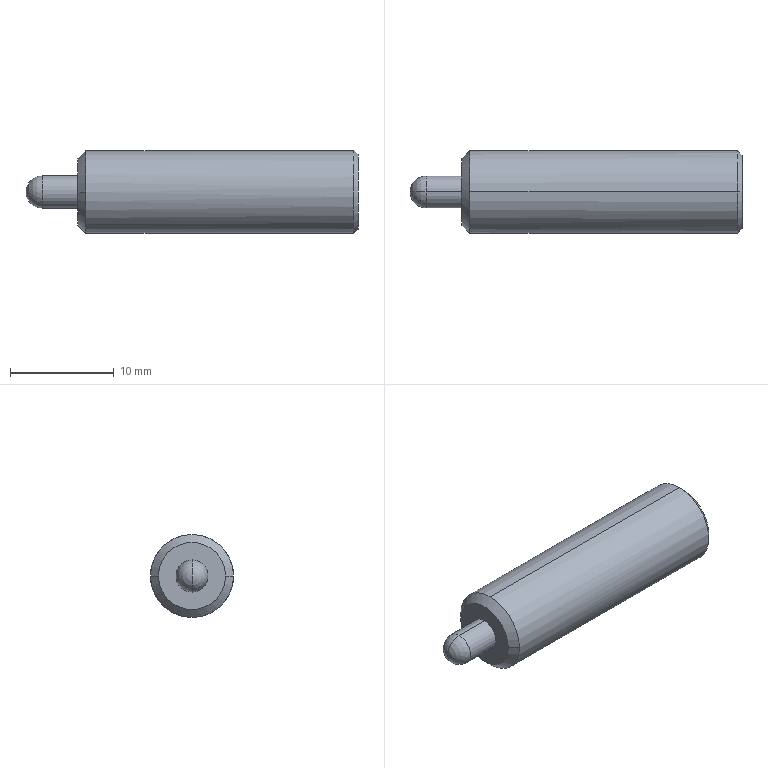Part | SolidWorks | features BaseBody 1 | 1 solid | 19 faces | box 32 x 8 x 8 mm | volume 1371 mm3 | plane 9 | cylinder 4 | cone 4 | sphere 2 | commonest cylinder face diameters 3.1 x2 8 x2
STEP:
#1=CARTESIAN_POINT('',(-3.45,0.,1.55));
#2=VERTEX_POINT('',#1);
#3=CARTESIAN_POINT('',(-3.45,0.,-1.55));
#4=VERTEX_POINT('',#3);
#5=CARTESIAN_POINT('',(-3.45,0.,0.));
#6=DIRECTION('',(1.,0.,0.));
#7=DIRECTION('',(0.,0.,-1.));
#8=AXIS2_PLACEMENT_3D('',#5,#6,#7);
#9=CIRCLE('',#8,1.55);
#10=EDGE_CURVE('',#2,#4,#9,.T.);
#11=ORIENTED_EDGE('',*,*,#10,.F.);
#12=CARTESIAN_POINT('',(-3.45,0.,0.));
#13=DIRECTION('',(0.,-1.,0.));
#14=DIRECTION('',(0.,0.,-1.));
#15=AXIS2_PLACEMENT_3D('',#12,#13,#14);
#16=CIRCLE('',#15,1.55);
#17=EDGE_CURVE('',#2,#4,#16,.T.);
#18=ORIENTED_EDGE('',*,*,#17,.T.);
#19=EDGE_LOOP('',(#11,#18));
#20=FACE_OUTER_BOUND('',#19,.T.);
#21=CARTESIAN_POINT('',(-3.45,0.,0.));
#22=DIRECTION('',(-1.,0.,0.));
#23=DIRECTION('',(0.,0.,-1.));
#24=AXIS2_PLACEMENT_3D('',#21,#22,#23);
#25=SPHERICAL_SURFACE('',#24,1.55);
#26=ADVANCED_FACE('',(#20),#25,.T.);
#27=CARTESIAN_POINT('',(27.,-0.7217,-1.25));
#28=VERTEX_POINT('',#27);
#29=CARTESIAN_POINT('',(25.,-0.7217,-1.25));
#30=VERTEX_POINT('',#29);
#31=CARTESIAN_POINT('',(25.,-0.7217,-1.25));
#32=DIRECTION('',(-1.,0.,0.));
#33=VECTOR('',#32,1000.);
#34=LINE('',#31,#33);
#35=EDGE_CURVE('',#28,#30,#34,.T.);
#36=ORIENTED_EDGE('',*,*,#35,.T.);
#37=CARTESIAN_POINT('',(25.,-1.443,0.));
#38=VERTEX_POINT('',#37);
#39=CARTESIAN_POINT('',(25.,-1.443,0.));
#40=DIRECTION('',(0.,0.5,-0.866));
#41=VECTOR('',#40,1000.);
#42=LINE('',#39,#41);
#43=EDGE_CURVE('',#38,#30,#42,.T.);
#44=ORIENTED_EDGE('',*,*,#43,.F.);
#45=CARTESIAN_POINT('',(27.,-1.443,0.));
#46=VERTEX_POINT('',#45);
#47=CARTESIAN_POINT('',(25.,-1.443,0.));
#48=DIRECTION('',(1.,0.,0.));
#49=VECTOR('',#48,1000.);
#50=LINE('',#47,#49);
#51=EDGE_CURVE('',#38,#46,#50,.T.);
#52=ORIENTED_EDGE('',*,*,#51,.T.);
#53=CARTESIAN_POINT('',(27.,-1.443,0.));
#54=DIRECTION('',(0.,-0.5,0.866));
#55=VECTOR('',#54,1000.);
#56=LINE('',#53,#55);
#57=EDGE_CURVE('',#28,#46,#56,.T.);
#58=ORIENTED_EDGE('',*,*,#57,.F.);
#59=EDGE_LOOP('',(#36,#44,#52,#58));
#60=FACE_OUTER_BOUND('',#59,.T.);
#61=CARTESIAN_POINT('',(25.,-1.443,0.));
#62=DIRECTION('',(0.,-0.866,-0.5));
#63=DIRECTION('',(0.,0.5,-0.866));
#64=AXIS2_PLACEMENT_3D('',#61,#62,#63);
#65=PLANE('',#64);
#66=ADVANCED_FACE('',(#60),#65,.F.);
#67=CARTESIAN_POINT('',(27.,0.7217,-1.25));
#68=VERTEX_POINT('',#67);
#69=CARTESIAN_POINT('',(25.,0.7217,-1.25));
#70=VERTEX_POINT('',#69);
#71=CARTESIAN_POINT('',(25.,0.7217,-1.25));
#72=DIRECTION('',(-1.,0.,0.));
#73=VECTOR('',#72,1000.);
#74=LINE('',#71,#73);
#75=EDGE_CURVE('',#68,#70,#74,.T.);
#76=ORIENTED_EDGE('',*,*,#75,.T.);
#77=CARTESIAN_POINT('',(25.,-0.7217,-1.25));
#78=DIRECTION('',(0.,1.,0.));
#79=VECTOR('',#78,1000.);
#80=LINE('',#77,#79);
#81=EDGE_CURVE('',#30,#70,#80,.T.);
#82=ORIENTED_EDGE('',*,*,#81,.F.);
#83=ORIENTED_EDGE('',*,*,#35,.F.);
#84=CARTESIAN_POINT('',(27.,-0.7217,-1.25));
#85=DIRECTION('',(0.,-1.,0.));
#86=VECTOR('',#85,1000.);
#87=LINE('',#84,#86);
#88=EDGE_CURVE('',#68,#28,#87,.T.);
#89=ORIENTED_EDGE('',*,*,#88,.F.);
#90=EDGE_LOOP('',(#76,#82,#83,#89));
#91=FACE_OUTER_BOUND('',#90,.T.);
#92=CARTESIAN_POINT('',(25.,-0.7217,-1.25));
#93=DIRECTION('',(0.,0.,-1.));
#94=DIRECTION('',(0.,-1.,0.));
#95=AXIS2_PLACEMENT_3D('',#92,#93,#94);
#96=PLANE('',#95);
#97=ADVANCED_FACE('',(#91),#96,.F.);
#98=ORIENTED_EDGE('',*,*,#51,.F.);
#99=CARTESIAN_POINT('',(25.,-0.7217,1.25));
#100=VERTEX_POINT('',#99);
#101=CARTESIAN_POINT('',(25.,-0.7217,1.25));
#102=DIRECTION('',(0.,-0.5,-0.866));
#103=VECTOR('',#102,1000.);
#104=LINE('',#101,#103);
#105=EDGE_CURVE('',#100,#38,#104,.T.);
#106=ORIENTED_EDGE('',*,*,#105,.F.);
#107=CARTESIAN_POINT('',(27.,-0.7217,1.25));
#108=VERTEX_POINT('',#107);
#109=CARTESIAN_POINT('',(25.,-0.7217,1.25));
#110=DIRECTION('',(1.,0.,0.));
#111=VECTOR('',#110,1000.);
#112=LINE('',#109,#111);
#113=EDGE_CURVE('',#100,#108,#112,.T.);
#114=ORIENTED_EDGE('',*,*,#113,.T.);
#115=CARTESIAN_POINT('',(27.,-0.7217,1.25));
#116=DIRECTION('',(0.,0.5,0.866));
#117=VECTOR('',#116,1000.);
#118=LINE('',#115,#117);
#119=EDGE_CURVE('',#46,#108,#118,.T.);
#120=ORIENTED_EDGE('',*,*,#119,.F.);
#121=EDGE_LOOP('',(#98,#106,#114,#120));
#122=FACE_OUTER_BOUND('',#121,.T.);
#123=CARTESIAN_POINT('',(25.,-0.7217,1.25));
#124=DIRECTION('',(0.,-0.866,0.5));
#125=DIRECTION('',(-1.,0.,0.));
#126=AXIS2_PLACEMENT_3D('',#123,#124,#125);
#127=PLANE('',#126);
#128=ADVANCED_FACE('',(#122),#127,.F.);
#129=CARTESIAN_POINT('',(27.,1.443,0.));
#130=VERTEX_POINT('',#129);
#131=CARTESIAN_POINT('',(25.,1.443,0.));
#132=VERTEX_POINT('',#131);
#133=CARTESIAN_POINT('',(25.,1.443,0.));
#134=DIRECTION('',(-1.,0.,0.));
#135=VECTOR('',#134,1000.);
#136=LINE('',#133,#135);
#137=EDGE_CURVE('',#130,#132,#136,.T.);
#138=ORIENTED_EDGE('',*,*,#137,.T.);
#139=CARTESIAN_POINT('',(25.,0.7217,-1.25));
#140=DIRECTION('',(0.,0.5,0.866));
#141=VECTOR('',#140,1000.);
#142=LINE('',#139,#141);
#143=EDGE_CURVE('',#70,#132,#142,.T.);
#144=ORIENTED_EDGE('',*,*,#143,.F.);
#145=ORIENTED_EDGE('',*,*,#75,.F.);
#146=CARTESIAN_POINT('',(27.,0.7217,-1.25));
#147=DIRECTION('',(0.,-0.5,-0.866));
#148=VECTOR('',#147,1000.);
#149=LINE('',#146,#148);
#150=EDGE_CURVE('',#130,#68,#149,.T.);
#151=ORIENTED_EDGE('',*,*,#150,.F.);
#152=EDGE_LOOP('',(#138,#144,#145,#151));
#153=FACE_OUTER_BOUND('',#152,.T.);
#154=CARTESIAN_POINT('',(25.,0.7217,-1.25));
#155=DIRECTION('',(0.,0.866,-0.5));
#156=DIRECTION('',(-1.,0.,0.));
#157=AXIS2_PLACEMENT_3D('',#154,#155,#156);
#158=PLANE('',#157);
#159=ADVANCED_FACE('',(#153),#158,.F.);
#160=ORIENTED_EDGE('',*,*,#143,.T.);
#161=CARTESIAN_POINT('',(25.,0.7217,1.25));
#162=VERTEX_POINT('',#161);
#163=CARTESIAN_POINT('',(25.,1.443,0.));
#164=DIRECTION('',(0.,-0.5,0.866));
#165=VECTOR('',#164,1000.);
#166=LINE('',#163,#165);
#167=EDGE_CURVE('',#132,#162,#166,.T.);
#168=ORIENTED_EDGE('',*,*,#167,.T.);
#169=CARTESIAN_POINT('',(25.,0.7217,1.25));
#170=DIRECTION('',(0.,-1.,0.));
#171=VECTOR('',#170,1000.);
#172=LINE('',#169,#171);
#173=EDGE_CURVE('',#162,#100,#172,.T.);
#174=ORIENTED_EDGE('',*,*,#173,.T.);
#175=ORIENTED_EDGE('',*,*,#105,.T.);
#176=ORIENTED_EDGE('',*,*,#43,.T.);
#177=ORIENTED_EDGE('',*,*,#81,.T.);
#178=EDGE_LOOP('',(#160,#168,#174,#175,#176,#177));
#179=FACE_OUTER_BOUND('',#178,.T.);
#180=CARTESIAN_POINT('',(25.,0.,0.));
#181=DIRECTION('',(1.,0.,0.));
#182=DIRECTION('',(0.,1.,0.));
#183=AXIS2_PLACEMENT_3D('',#180,#181,#182);
#184=PLANE('',#183);
#185=ADVANCED_FACE('',(#179),#184,.T.);
#186=ORIENTED_EDGE('',*,*,#113,.F.);
#187=ORIENTED_EDGE('',*,*,#173,.F.);
#188=CARTESIAN_POINT('',(27.,0.7217,1.25));
#189=VERTEX_POINT('',#188);
#190=CARTESIAN_POINT('',(25.,0.7217,1.25));
#191=DIRECTION('',(1.,0.,0.));
#192=VECTOR('',#191,1000.);
#193=LINE('',#190,#192);
#194=EDGE_CURVE('',#162,#189,#193,.T.);
#195=ORIENTED_EDGE('',*,*,#194,.T.);
#196=CARTESIAN_POINT('',(27.,0.7217,1.25));
#197=DIRECTION('',(0.,1.,0.));
#198=VECTOR('',#197,1000.);
#199=LINE('',#196,#198);
#200=EDGE_CURVE('',#108,#189,#199,.T.);
#201=ORIENTED_EDGE('',*,*,#200,.F.);
#202=EDGE_LOOP('',(#186,#187,#195,#201));
#203=FACE_OUTER_BOUND('',#202,.T.);
#204=CARTESIAN_POINT('',(25.,0.7217,1.25));
#205=DIRECTION('',(0.,0.,1.));
#206=DIRECTION('',(1.,0.,0.));
#207=AXIS2_PLACEMENT_3D('',#204,#205,#206);
#208=PLANE('',#207);
#209=ADVANCED_FACE('',(#203),#208,.F.);
#210=ORIENTED_EDGE('',*,*,#194,.F.);
#211=ORIENTED_EDGE('',*,*,#167,.F.);
#212=ORIENTED_EDGE('',*,*,#137,.F.);
#213=CARTESIAN_POINT('',(27.,1.443,0.));
#214=DIRECTION('',(0.,-0.5,0.866));
#215=VECTOR('',#214,1000.);
#216=LINE('',#213,#215);
#217=EDGE_CURVE('',#130,#189,#216,.T.);
#218=ORIENTED_EDGE('',*,*,#217,.T.);
#219=EDGE_LOOP('',(#210,#211,#212,#218));
#220=FACE_OUTER_BOUND('',#219,.T.);
#221=CARTESIAN_POINT('',(25.,1.443,0.));
#222=DIRECTION('',(0.,0.866,0.5));
#223=DIRECTION('',(1.,0.,0.));
#224=AXIS2_PLACEMENT_3D('',#221,#222,#223);
#225=PLANE('',#224);
#226=ADVANCED_FACE('',(#220),#225,.F.);
#227=CARTESIAN_POINT('',(0.,0.,-1.55));
#228=VERTEX_POINT('',#227);
#229=CARTESIAN_POINT('',(54.,0.,-1.55));
#230=DIRECTION('',(-1.,0.,0.));
#231=VECTOR('',#230,1000.);
#232=LINE('',#229,#231);
#233=EDGE_CURVE('',#228,#4,#232,.T.);
#234=ORIENTED_EDGE('',*,*,#233,.F.);
#235=CARTESIAN_POINT('',(0.,0.,1.55));
#236=VERTEX_POINT('',#235);
#237=CARTESIAN_POINT('',(0.,0.,0.));
#238=DIRECTION('',(-1.,0.,0.));
#239=DIRECTION('',(0.,0.,1.));
#240=AXIS2_PLACEMENT_3D('',#237,#238,#239);
#241=CIRCLE('',#240,1.55);
#242=EDGE_CURVE('',#228,#236,#241,.T.);
#243=ORIENTED_EDGE('',*,*,#242,.T.);
#244=CARTESIAN_POINT('',(54.,0.,1.55));
#245=DIRECTION('',(-1.,0.,0.));
#246=VECTOR('',#245,1000.);
#247=LINE('',#244,#246);
#248=EDGE_CURVE('',#236,#2,#247,.T.);
#249=ORIENTED_EDGE('',*,*,#248,.T.);
#250=ORIENTED_EDGE('',*,*,#10,.T.);
#251=EDGE_LOOP('',(#234,#243,#249,#250));
#252=FACE_OUTER_BOUND('',#251,.T.);
#253=CARTESIAN_POINT('',(54.,0.,0.));
#254=DIRECTION('',(-1.,0.,0.));
#255=DIRECTION('',(0.,0.,1.));
#256=AXIS2_PLACEMENT_3D('',#253,#254,#255);
#257=CYLINDRICAL_SURFACE('',#256,1.55);
#258=ADVANCED_FACE('',(#252),#257,.T.);
#259=ORIENTED_EDGE('',*,*,#150,.T.);
#260=ORIENTED_EDGE('',*,*,#88,.T.);
#261=ORIENTED_EDGE('',*,*,#57,.T.);
#262=ORIENTED_EDGE('',*,*,#119,.T.);
#263=ORIENTED_EDGE('',*,*,#200,.T.);
#264=ORIENTED_EDGE('',*,*,#217,.F.);
#265=EDGE_LOOP('',(#259,#260,#261,#262,#263,#264));
#266=FACE_BOUND('',#265,.T.);
#267=CARTESIAN_POINT('',(27.,0.,3.576));
#268=VERTEX_POINT('',#267);
#269=CARTESIAN_POINT('',(27.,0.,-3.576));
#270=VERTEX_POINT('',#269);
#271=CARTESIAN_POINT('',(27.,0.,0.));
#272=DIRECTION('',(-1.,0.,0.));
#273=DIRECTION('',(0.,0.,1.));
#274=AXIS2_PLACEMENT_3D('',#271,#272,#273);
#275=CIRCLE('',#274,3.576);
#276=EDGE_CURVE('',#268,#270,#275,.T.);
#277=ORIENTED_EDGE('',*,*,#276,.F.);
#278=CARTESIAN_POINT('',(27.,0.,0.));
#279=DIRECTION('',(-1.,0.,0.));
#280=DIRECTION('',(0.,0.,1.));
#281=AXIS2_PLACEMENT_3D('',#278,#279,#280);
#282=CIRCLE('',#281,3.576);
#283=EDGE_CURVE('',#270,#268,#282,.T.);
#284=ORIENTED_EDGE('',*,*,#283,.F.);
#285=EDGE_LOOP('',(#277,#284));
#286=FACE_OUTER_BOUND('',#285,.T.);
#287=CARTESIAN_POINT('',(27.,3.576,0.));
#288=DIRECTION('',(-1.,0.,0.));
#289=DIRECTION('',(0.,0.,1.));
#290=AXIS2_PLACEMENT_3D('',#287,#288,#289);
#291=PLANE('',#290);
#292=ADVANCED_FACE('',(#266,#286),#291,.F.);
#293=CARTESIAN_POINT('',(0.,0.,0.));
#294=DIRECTION('',(-1.,0.,0.));
#295=DIRECTION('',(0.,0.,1.));
#296=AXIS2_PLACEMENT_3D('',#293,#294,#295);
#297=CIRCLE('',#296,1.55);
#298=EDGE_CURVE('',#236,#228,#297,.T.);
#299=ORIENTED_EDGE('',*,*,#298,.F.);
#300=ORIENTED_EDGE('',*,*,#242,.F.);
#301=EDGE_LOOP('',(#299,#300));
#302=FACE_BOUND('',#301,.T.);
#303=CARTESIAN_POINT('',(0.,3.233,0.));
#304=VERTEX_POINT('',#303);
#305=CARTESIAN_POINT('',(0.,-3.233,0.));
#306=VERTEX_POINT('',#305);
#307=CARTESIAN_POINT('',(0.,0.,0.));
#308=DIRECTION('',(1.,0.,0.));
#309=DIRECTION('',(0.,1.,0.));
#310=AXIS2_PLACEMENT_3D('',#307,#308,#309);
#311=CIRCLE('',#310,3.233);
#312=EDGE_CURVE('',#304,#306,#311,.T.);
#313=ORIENTED_EDGE('',*,*,#312,.F.);
#314=CARTESIAN_POINT('',(0.,0.,0.));
#315=DIRECTION('',(1.,0.,0.));
#316=DIRECTION('',(0.,1.,0.));
#317=AXIS2_PLACEMENT_3D('',#314,#315,#316);
#318=CIRCLE('',#317,3.233);
#319=EDGE_CURVE('',#306,#304,#318,.T.);
#320=ORIENTED_EDGE('',*,*,#319,.F.);
#321=EDGE_LOOP('',(#313,#320));
#322=FACE_OUTER_BOUND('',#321,.T.);
#323=CARTESIAN_POINT('',(0.,1.55,0.));
#324=DIRECTION('',(1.,0.,0.));
#325=DIRECTION('',(0.,1.,0.));
#326=AXIS2_PLACEMENT_3D('',#323,#324,#325);
#327=PLANE('',#326);
#328=ADVANCED_FACE('',(#302,#322),#327,.F.);
#329=CARTESIAN_POINT('',(26.576,0.,-4.));
#330=VERTEX_POINT('',#329);
#331=CARTESIAN_POINT('',(26.576,0.,-4.));
#332=DIRECTION('',(-0.7071,0.,-0.7071));
#333=VECTOR('',#332,1000.);
#334=LINE('',#331,#333);
#335=EDGE_CURVE('',#270,#330,#334,.T.);
#336=ORIENTED_EDGE('',*,*,#335,.F.);
#337=ORIENTED_EDGE('',*,*,#283,.T.);
#338=CARTESIAN_POINT('',(26.576,0.,4.));
#339=VERTEX_POINT('',#338);
#340=CARTESIAN_POINT('',(26.576,0.,4.));
#341=DIRECTION('',(-0.7071,0.,0.7071));
#342=VECTOR('',#341,1000.);
#343=LINE('',#340,#342);
#344=EDGE_CURVE('',#268,#339,#343,.T.);
#345=ORIENTED_EDGE('',*,*,#344,.T.);
#346=CARTESIAN_POINT('',(26.576,0.,0.));
#347=DIRECTION('',(-1.,0.,0.));
#348=DIRECTION('',(0.,0.,1.));
#349=AXIS2_PLACEMENT_3D('',#346,#347,#348);
#350=CIRCLE('',#349,4.);
#351=EDGE_CURVE('',#330,#339,#350,.T.);
#352=ORIENTED_EDGE('',*,*,#351,.F.);
#353=EDGE_LOOP('',(#336,#337,#345,#352));
#354=FACE_OUTER_BOUND('',#353,.T.);
#355=CARTESIAN_POINT('',(26.576,0.,0.));
#356=DIRECTION('',(-1.,0.,0.));
#357=DIRECTION('',(0.,0.,1.));
#358=AXIS2_PLACEMENT_3D('',#355,#356,#357);
#359=CONICAL_SURFACE('',#358,4.,0.7854);
#360=ADVANCED_FACE('',(#354),#359,.T.);
#361=CARTESIAN_POINT('',(0.767,-4.,0.));
#362=VERTEX_POINT('',#361);
#363=CARTESIAN_POINT('',(0.767,-4.,0.));
#364=DIRECTION('',(0.7071,-0.7071,0.));
#365=VECTOR('',#364,1000.);
#366=LINE('',#363,#365);
#367=EDGE_CURVE('',#306,#362,#366,.T.);
#368=ORIENTED_EDGE('',*,*,#367,.F.);
#369=ORIENTED_EDGE('',*,*,#319,.T.);
#370=CARTESIAN_POINT('',(0.767,4.,0.));
#371=VERTEX_POINT('',#370);
#372=CARTESIAN_POINT('',(0.767,4.,0.));
#373=DIRECTION('',(0.7071,0.7071,0.));
#374=VECTOR('',#373,1000.);
#375=LINE('',#372,#374);
#376=EDGE_CURVE('',#304,#371,#375,.T.);
#377=ORIENTED_EDGE('',*,*,#376,.T.);
#378=CARTESIAN_POINT('',(0.767,0.,-4.));
#379=VERTEX_POINT('',#378);
#380=CARTESIAN_POINT('',(0.767,0.,0.));
#381=DIRECTION('',(1.,0.,0.));
#382=DIRECTION('',(0.,0.,1.));
#383=AXIS2_PLACEMENT_3D('',#380,#381,#382);
#384=CIRCLE('',#383,4.);
#385=EDGE_CURVE('',#379,#371,#384,.T.);
#386=ORIENTED_EDGE('',*,*,#385,.F.);
#387=CARTESIAN_POINT('',(0.767,0.,0.));
#388=DIRECTION('',(1.,0.,0.));
#389=DIRECTION('',(0.,0.,1.));
#390=AXIS2_PLACEMENT_3D('',#387,#388,#389);
#391=CIRCLE('',#390,4.);
#392=EDGE_CURVE('',#362,#379,#391,.T.);
#393=ORIENTED_EDGE('',*,*,#392,.F.);
#394=EDGE_LOOP('',(#368,#369,#377,#386,#393));
#395=FACE_OUTER_BOUND('',#394,.T.);
#396=CARTESIAN_POINT('',(0.767,0.,0.));
#397=DIRECTION('',(1.,0.,0.));
#398=DIRECTION('',(0.,1.,0.));
#399=AXIS2_PLACEMENT_3D('',#396,#397,#398);
#400=CONICAL_SURFACE('',#399,4.,0.7854);
#401=ADVANCED_FACE('',(#395),#400,.T.);
#402=CARTESIAN_POINT('',(54.,0.,-4.));
#403=DIRECTION('',(-1.,0.,0.));
#404=VECTOR('',#403,1000.);
#405=LINE('',#402,#404);
#406=EDGE_CURVE('',#330,#379,#405,.T.);
#407=ORIENTED_EDGE('',*,*,#406,.F.);
#408=ORIENTED_EDGE('',*,*,#351,.T.);
#409=CARTESIAN_POINT('',(0.767,0.,4.));
#410=VERTEX_POINT('',#409);
#411=CARTESIAN_POINT('',(54.,0.,4.));
#412=DIRECTION('',(-1.,0.,0.));
#413=VECTOR('',#412,1000.);
#414=LINE('',#411,#413);
#415=EDGE_CURVE('',#339,#410,#414,.T.);
#416=ORIENTED_EDGE('',*,*,#415,.T.);
#417=CARTESIAN_POINT('',(0.767,0.,0.));
#418=DIRECTION('',(1.,0.,0.));
#419=DIRECTION('',(0.,0.,1.));
#420=AXIS2_PLACEMENT_3D('',#417,#418,#419);
#421=CIRCLE('',#420,4.);
#422=EDGE_CURVE('',#410,#362,#421,.T.);
#423=ORIENTED_EDGE('',*,*,#422,.T.);
#424=ORIENTED_EDGE('',*,*,#392,.T.);
#425=EDGE_LOOP('',(#407,#408,#416,#423,#424));
#426=FACE_OUTER_BOUND('',#425,.T.);
#427=CARTESIAN_POINT('',(54.,0.,0.));
#428=DIRECTION('',(-1.,0.,0.));
#429=DIRECTION('',(0.,0.,1.));
#430=AXIS2_PLACEMENT_3D('',#427,#428,#429);
#431=CYLINDRICAL_SURFACE('',#430,4.);
#432=ADVANCED_FACE('',(#426),#431,.T.);
#433=ORIENTED_EDGE('',*,*,#298,.T.);
#434=ORIENTED_EDGE('',*,*,#233,.T.);
#435=CARTESIAN_POINT('',(-3.45,0.,0.));
#436=DIRECTION('',(1.,0.,0.));
#437=DIRECTION('',(0.,0.,-1.));
#438=AXIS2_PLACEMENT_3D('',#435,#436,#437);
#439=CIRCLE('',#438,1.55);
#440=EDGE_CURVE('',#4,#2,#439,.T.);
#441=ORIENTED_EDGE('',*,*,#440,.T.);
#442=ORIENTED_EDGE('',*,*,#248,.F.);
#443=EDGE_LOOP('',(#433,#434,#441,#442));
#444=FACE_OUTER_BOUND('',#443,.T.);
#445=CARTESIAN_POINT('',(54.,0.,0.));
#446=DIRECTION('',(-1.,0.,0.));
#447=DIRECTION('',(0.,0.,1.));
#448=AXIS2_PLACEMENT_3D('',#445,#446,#447);
#449=CYLINDRICAL_SURFACE('',#448,1.55);
#450=ADVANCED_FACE('',(#444),#449,.T.);
#451=ORIENTED_EDGE('',*,*,#276,.T.);
#452=ORIENTED_EDGE('',*,*,#335,.T.);
#453=CARTESIAN_POINT('',(26.576,0.,0.));
#454=DIRECTION('',(-1.,0.,0.));
#455=DIRECTION('',(0.,0.,1.));
#456=AXIS2_PLACEMENT_3D('',#453,#454,#455);
#457=CIRCLE('',#456,4.);
#458=EDGE_CURVE('',#339,#330,#457,.T.);
#459=ORIENTED_EDGE('',*,*,#458,.F.);
#460=ORIENTED_EDGE('',*,*,#344,.F.);
#461=EDGE_LOOP('',(#451,#452,#459,#460));
#462=FACE_OUTER_BOUND('',#461,.T.);
#463=CARTESIAN_POINT('',(26.576,0.,0.));
#464=DIRECTION('',(-1.,0.,0.));
#465=DIRECTION('',(0.,0.,1.));
#466=AXIS2_PLACEMENT_3D('',#463,#464,#465);
#467=CONICAL_SURFACE('',#466,4.,0.7854);
#468=ADVANCED_FACE('',(#462),#467,.T.);
#469=ORIENTED_EDGE('',*,*,#312,.T.);
#470=ORIENTED_EDGE('',*,*,#367,.T.);
#471=ORIENTED_EDGE('',*,*,#422,.F.);
#472=CARTESIAN_POINT('',(0.767,0.,0.));
#473=DIRECTION('',(1.,0.,0.));
#474=DIRECTION('',(0.,0.,1.));
#475=AXIS2_PLACEMENT_3D('',#472,#473,#474);
#476=CIRCLE('',#475,4.);
#477=EDGE_CURVE('',#371,#410,#476,.T.);
#478=ORIENTED_EDGE('',*,*,#477,.F.);
#479=ORIENTED_EDGE('',*,*,#376,.F.);
#480=EDGE_LOOP('',(#469,#470,#471,#478,#479));
#481=FACE_OUTER_BOUND('',#480,.T.);
#482=CARTESIAN_POINT('',(0.767,0.,0.));
#483=DIRECTION('',(1.,0.,0.));
#484=DIRECTION('',(0.,1.,0.));
#485=AXIS2_PLACEMENT_3D('',#482,#483,#484);
#486=CONICAL_SURFACE('',#485,4.,0.7854);
#487=ADVANCED_FACE('',(#481),#486,.T.);
#488=ORIENTED_EDGE('',*,*,#458,.T.);
#489=ORIENTED_EDGE('',*,*,#406,.T.);
#490=ORIENTED_EDGE('',*,*,#385,.T.);
#491=ORIENTED_EDGE('',*,*,#477,.T.);
#492=ORIENTED_EDGE('',*,*,#415,.F.);
#493=EDGE_LOOP('',(#488,#489,#490,#491,#492));
#494=FACE_OUTER_BOUND('',#493,.T.);
#495=CARTESIAN_POINT('',(54.,0.,0.));
#496=DIRECTION('',(-1.,0.,0.));
#497=DIRECTION('',(0.,0.,1.));
#498=AXIS2_PLACEMENT_3D('',#495,#496,#497);
#499=CYLINDRICAL_SURFACE('',#498,4.);
#500=ADVANCED_FACE('',(#494),#499,.T.);
#501=ORIENTED_EDGE('',*,*,#17,.F.);
#502=ORIENTED_EDGE('',*,*,#440,.F.);
#503=EDGE_LOOP('',(#501,#502));
#504=FACE_OUTER_BOUND('',#503,.T.);
#505=CARTESIAN_POINT('',(-3.45,0.,0.));
#506=DIRECTION('',(-1.,0.,0.));
#507=DIRECTION('',(0.,0.,-1.));
#508=AXIS2_PLACEMENT_3D('',#505,#506,#507);
#509=SPHERICAL_SURFACE('',#508,1.55);
#510=ADVANCED_FACE('',(#504),#509,.T.);
#511=CLOSED_SHELL('',(#26,#66,#97,#128,#159,#185,#209,#226,#258,#292,#328,#360,#401,#432,#450,#468,#487,#500,#510));
#512=MANIFOLD_SOLID_BREP('',#511);
#513=CARTESIAN_POINT('',(0.,0.,0.));
#514=DIRECTION('',(0.,0.,1.));
#515=DIRECTION('',(1.,0.,0.));
#516=AXIS2_PLACEMENT_3D('',#513,#514,#515);
#517=(LENGTH_UNIT()NAMED_UNIT(*)SI_UNIT(.MILLI.,.METRE.));
#518=UNCERTAINTY_MEASURE_WITH_UNIT(LENGTH_MEASURE(0.00001),#517,'','');
#519=(NAMED_UNIT(*)PLANE_ANGLE_UNIT()SI_UNIT($,.RADIAN.));
#520=(NAMED_UNIT(*)SI_UNIT($,.STERADIAN.)SOLID_ANGLE_UNIT());
#521=(GEOMETRIC_REPRESENTATION_CONTEXT(3)GLOBAL_UNCERTAINTY_ASSIGNED_CONTEXT((#518))GLOBAL_UNIT_ASSIGNED_CONTEXT((#517,#519,#520))REPRESENTATION_CONTEXT('',''));
#522=ADVANCED_BREP_SHAPE_REPRESENTATION('',(#512,#516),#521);